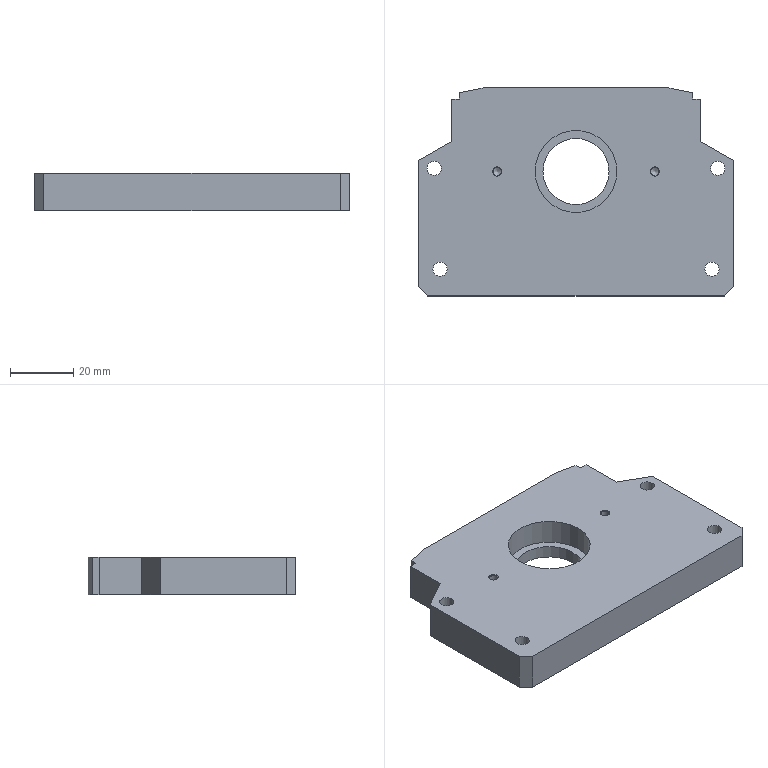Part | NX | 1 solid | 45 faces | box 100 x 66 x 12 mm | volume 66555 mm3 | plane 23 | cylinder 14 | cone 8 | commonest cylinder face diameters 2.5 x4 4.5 x4 8 x4 21 x1 26 x1
STEP:
#1=CARTESIAN_POINT('',(569.577,189.79,0.));
#2=VERTEX_POINT('',#1);
#3=CARTESIAN_POINT('',(559.077,189.79,0.));
#4=DIRECTION('',(0.,0.,-1.));
#5=DIRECTION('',(1.,0.,0.));
#6=AXIS2_PLACEMENT_3D('',#3,#4,#5);
#7=CIRCLE('',#6,10.5);
#8=EDGE_CURVE('',#2,#2,#7,.T.);
#9=ORIENTED_EDGE('',*,*,#8,.T.);
#10=EDGE_LOOP('',(#9));
#11=FACE_BOUND('',#10,.T.);
#12=CARTESIAN_POINT('',(569.577,189.79,4.));
#13=VERTEX_POINT('',#12);
#14=CARTESIAN_POINT('',(559.077,189.79,4.));
#15=DIRECTION('',(0.,0.,1.));
#16=DIRECTION('',(1.,0.,0.));
#17=AXIS2_PLACEMENT_3D('',#14,#15,#16);
#18=CIRCLE('',#17,10.5);
#19=EDGE_CURVE('',#13,#13,#18,.T.);
#20=ORIENTED_EDGE('',*,*,#19,.T.);
#21=EDGE_LOOP('',(#20));
#22=FACE_BOUND('',#21,.T.);
#23=CARTESIAN_POINT('',(559.077,189.79,0.));
#24=DIRECTION('',(0.,0.,1.));
#25=DIRECTION('',(-1.,0.,0.));
#26=AXIS2_PLACEMENT_3D('',#23,#24,#25);
#27=CYLINDRICAL_SURFACE('',#26,10.5);
#28=ADVANCED_FACE('',(#11,#22),#27,.F.);
#29=CARTESIAN_POINT('',(509.077,193.29,12.));
#30=VERTEX_POINT('',#29);
#31=CARTESIAN_POINT('',(509.077,153.29,12.));
#32=VERTEX_POINT('',#31);
#33=CARTESIAN_POINT('',(509.077,193.29,12.));
#34=DIRECTION('',(0.,-1.,0.));
#35=VECTOR('',#34,1.);
#36=LINE('',#33,#35);
#37=EDGE_CURVE('',#30,#32,#36,.T.);
#38=ORIENTED_EDGE('',*,*,#37,.F.);
#39=CARTESIAN_POINT('',(509.077,193.29,0.));
#40=VERTEX_POINT('',#39);
#41=CARTESIAN_POINT('',(509.077,193.29,0.));
#42=DIRECTION('',(0.,0.,1.));
#43=VECTOR('',#42,1.);
#44=LINE('',#41,#43);
#45=EDGE_CURVE('',#40,#30,#44,.T.);
#46=ORIENTED_EDGE('',*,*,#45,.F.);
#47=CARTESIAN_POINT('',(509.077,153.29,0.));
#48=VERTEX_POINT('',#47);
#49=CARTESIAN_POINT('',(509.077,193.29,0.));
#50=DIRECTION('',(0.,-1.,0.));
#51=VECTOR('',#50,1.);
#52=LINE('',#49,#51);
#53=EDGE_CURVE('',#40,#48,#52,.T.);
#54=ORIENTED_EDGE('',*,*,#53,.T.);
#55=CARTESIAN_POINT('',(509.077,153.29,0.));
#56=DIRECTION('',(0.,0.,1.));
#57=VECTOR('',#56,1.);
#58=LINE('',#55,#57);
#59=EDGE_CURVE('',#48,#32,#58,.T.);
#60=ORIENTED_EDGE('',*,*,#59,.T.);
#61=EDGE_LOOP('',(#38,#46,#54,#60));
#62=FACE_OUTER_BOUND('',#61,.T.);
#63=CARTESIAN_POINT('',(509.077,193.29,0.));
#64=DIRECTION('',(-1.,0.,0.));
#65=DIRECTION('',(0.,0.,-1.));
#66=AXIS2_PLACEMENT_3D('',#63,#64,#65);
#67=PLANE('',#66);
#68=ADVANCED_FACE('',(#62),#67,.T.);
#69=CARTESIAN_POINT('',(512.077,150.29,12.));
#70=VERTEX_POINT('',#69);
#71=CARTESIAN_POINT('',(509.077,153.29,12.));
#72=DIRECTION('',(0.7071,-0.7071,0.));
#73=VECTOR('',#72,1.);
#74=LINE('',#71,#73);
#75=EDGE_CURVE('',#32,#70,#74,.T.);
#76=ORIENTED_EDGE('',*,*,#75,.F.);
#77=ORIENTED_EDGE('',*,*,#59,.F.);
#78=CARTESIAN_POINT('',(512.077,150.29,0.));
#79=VERTEX_POINT('',#78);
#80=CARTESIAN_POINT('',(509.077,153.29,0.));
#81=DIRECTION('',(0.7071,-0.7071,0.));
#82=VECTOR('',#81,1.);
#83=LINE('',#80,#82);
#84=EDGE_CURVE('',#48,#79,#83,.T.);
#85=ORIENTED_EDGE('',*,*,#84,.T.);
#86=CARTESIAN_POINT('',(512.077,150.29,0.));
#87=DIRECTION('',(0.,0.,1.));
#88=VECTOR('',#87,1.);
#89=LINE('',#86,#88);
#90=EDGE_CURVE('',#79,#70,#89,.T.);
#91=ORIENTED_EDGE('',*,*,#90,.T.);
#92=EDGE_LOOP('',(#76,#77,#85,#91));
#93=FACE_OUTER_BOUND('',#92,.T.);
#94=CARTESIAN_POINT('',(509.077,153.29,0.));
#95=DIRECTION('',(-0.7071,-0.7071,0.));
#96=DIRECTION('',(-0.7071,0.7071,0.));
#97=AXIS2_PLACEMENT_3D('',#94,#95,#96);
#98=PLANE('',#97);
#99=ADVANCED_FACE('',(#93),#98,.T.);
#100=CARTESIAN_POINT('',(606.077,150.29,12.));
#101=VERTEX_POINT('',#100);
#102=CARTESIAN_POINT('',(512.077,150.29,12.));
#103=DIRECTION('',(1.,0.,0.));
#104=VECTOR('',#103,1.);
#105=LINE('',#102,#104);
#106=EDGE_CURVE('',#70,#101,#105,.T.);
#107=ORIENTED_EDGE('',*,*,#106,.F.);
#108=ORIENTED_EDGE('',*,*,#90,.F.);
#109=CARTESIAN_POINT('',(606.077,150.29,0.));
#110=VERTEX_POINT('',#109);
#111=CARTESIAN_POINT('',(512.077,150.29,0.));
#112=DIRECTION('',(1.,0.,0.));
#113=VECTOR('',#112,1.);
#114=LINE('',#111,#113);
#115=EDGE_CURVE('',#79,#110,#114,.T.);
#116=ORIENTED_EDGE('',*,*,#115,.T.);
#117=CARTESIAN_POINT('',(606.077,150.29,0.));
#118=DIRECTION('',(0.,0.,1.));
#119=VECTOR('',#118,1.);
#120=LINE('',#117,#119);
#121=EDGE_CURVE('',#110,#101,#120,.T.);
#122=ORIENTED_EDGE('',*,*,#121,.T.);
#123=EDGE_LOOP('',(#107,#108,#116,#122));
#124=FACE_OUTER_BOUND('',#123,.T.);
#125=CARTESIAN_POINT('',(512.077,150.29,0.));
#126=DIRECTION('',(0.,-1.,0.));
#127=DIRECTION('',(0.,0.,1.));
#128=AXIS2_PLACEMENT_3D('',#125,#126,#127);
#129=PLANE('',#128);
#130=ADVANCED_FACE('',(#124),#129,.T.);
#131=CARTESIAN_POINT('',(609.077,153.29,12.));
#132=VERTEX_POINT('',#131);
#133=CARTESIAN_POINT('',(606.077,150.29,12.));
#134=DIRECTION('',(0.7071,0.7071,0.));
#135=VECTOR('',#134,1.);
#136=LINE('',#133,#135);
#137=EDGE_CURVE('',#101,#132,#136,.T.);
#138=ORIENTED_EDGE('',*,*,#137,.F.);
#139=ORIENTED_EDGE('',*,*,#121,.F.);
#140=CARTESIAN_POINT('',(609.077,153.29,0.));
#141=VERTEX_POINT('',#140);
#142=CARTESIAN_POINT('',(606.077,150.29,0.));
#143=DIRECTION('',(0.7071,0.7071,0.));
#144=VECTOR('',#143,1.);
#145=LINE('',#142,#144);
#146=EDGE_CURVE('',#110,#141,#145,.T.);
#147=ORIENTED_EDGE('',*,*,#146,.T.);
#148=CARTESIAN_POINT('',(609.077,153.29,0.));
#149=DIRECTION('',(0.,0.,1.));
#150=VECTOR('',#149,1.);
#151=LINE('',#148,#150);
#152=EDGE_CURVE('',#141,#132,#151,.T.);
#153=ORIENTED_EDGE('',*,*,#152,.T.);
#154=EDGE_LOOP('',(#138,#139,#147,#153));
#155=FACE_OUTER_BOUND('',#154,.T.);
#156=CARTESIAN_POINT('',(606.077,150.29,0.));
#157=DIRECTION('',(0.7071,-0.7071,0.));
#158=DIRECTION('',(-0.7071,-0.7071,0.));
#159=AXIS2_PLACEMENT_3D('',#156,#157,#158);
#160=PLANE('',#159);
#161=ADVANCED_FACE('',(#155),#160,.T.);
#162=CARTESIAN_POINT('',(609.077,193.29,12.));
#163=VERTEX_POINT('',#162);
#164=CARTESIAN_POINT('',(609.077,153.29,12.));
#165=DIRECTION('',(0.,1.,0.));
#166=VECTOR('',#165,1.);
#167=LINE('',#164,#166);
#168=EDGE_CURVE('',#132,#163,#167,.T.);
#169=ORIENTED_EDGE('',*,*,#168,.F.);
#170=ORIENTED_EDGE('',*,*,#152,.F.);
#171=CARTESIAN_POINT('',(609.077,193.29,0.));
#172=VERTEX_POINT('',#171);
#173=CARTESIAN_POINT('',(609.077,153.29,0.));
#174=DIRECTION('',(0.,1.,0.));
#175=VECTOR('',#174,1.);
#176=LINE('',#173,#175);
#177=EDGE_CURVE('',#141,#172,#176,.T.);
#178=ORIENTED_EDGE('',*,*,#177,.T.);
#179=CARTESIAN_POINT('',(609.077,193.29,0.));
#180=DIRECTION('',(0.,0.,1.));
#181=VECTOR('',#180,1.);
#182=LINE('',#179,#181);
#183=EDGE_CURVE('',#172,#163,#182,.T.);
#184=ORIENTED_EDGE('',*,*,#183,.T.);
#185=EDGE_LOOP('',(#169,#170,#178,#184));
#186=FACE_OUTER_BOUND('',#185,.T.);
#187=CARTESIAN_POINT('',(609.077,153.29,0.));
#188=DIRECTION('',(1.,0.,0.));
#189=DIRECTION('',(0.,0.,1.));
#190=AXIS2_PLACEMENT_3D('',#187,#188,#189);
#191=PLANE('',#190);
#192=ADVANCED_FACE('',(#186),#191,.T.);
#193=CARTESIAN_POINT('',(598.577,199.29,12.));
#194=VERTEX_POINT('',#193);
#195=CARTESIAN_POINT('',(609.077,193.29,12.));
#196=DIRECTION('',(-0.8682,0.4961,0.));
#197=VECTOR('',#196,1.);
#198=LINE('',#195,#197);
#199=EDGE_CURVE('',#163,#194,#198,.T.);
#200=ORIENTED_EDGE('',*,*,#199,.F.);
#201=ORIENTED_EDGE('',*,*,#183,.F.);
#202=CARTESIAN_POINT('',(598.577,199.29,0.));
#203=VERTEX_POINT('',#202);
#204=CARTESIAN_POINT('',(609.077,193.29,0.));
#205=DIRECTION('',(-0.8682,0.4961,0.));
#206=VECTOR('',#205,1.);
#207=LINE('',#204,#206);
#208=EDGE_CURVE('',#172,#203,#207,.T.);
#209=ORIENTED_EDGE('',*,*,#208,.T.);
#210=CARTESIAN_POINT('',(598.577,199.29,0.));
#211=DIRECTION('',(0.,0.,1.));
#212=VECTOR('',#211,1.);
#213=LINE('',#210,#212);
#214=EDGE_CURVE('',#203,#194,#213,.T.);
#215=ORIENTED_EDGE('',*,*,#214,.T.);
#216=EDGE_LOOP('',(#200,#201,#209,#215));
#217=FACE_OUTER_BOUND('',#216,.T.);
#218=CARTESIAN_POINT('',(609.077,193.29,0.));
#219=DIRECTION('',(0.4961,0.8682,0.));
#220=DIRECTION('',(0.8682,-0.4961,0.));
#221=AXIS2_PLACEMENT_3D('',#218,#219,#220);
#222=PLANE('',#221);
#223=ADVANCED_FACE('',(#217),#222,.T.);
#224=CARTESIAN_POINT('',(598.577,212.79,12.));
#225=VERTEX_POINT('',#224);
#226=CARTESIAN_POINT('',(598.577,199.29,12.));
#227=DIRECTION('',(0.,1.,0.));
#228=VECTOR('',#227,1.);
#229=LINE('',#226,#228);
#230=EDGE_CURVE('',#194,#225,#229,.T.);
#231=ORIENTED_EDGE('',*,*,#230,.F.);
#232=ORIENTED_EDGE('',*,*,#214,.F.);
#233=CARTESIAN_POINT('',(598.577,212.79,0.));
#234=VERTEX_POINT('',#233);
#235=CARTESIAN_POINT('',(598.577,199.29,0.));
#236=DIRECTION('',(0.,1.,0.));
#237=VECTOR('',#236,1.);
#238=LINE('',#235,#237);
#239=EDGE_CURVE('',#203,#234,#238,.T.);
#240=ORIENTED_EDGE('',*,*,#239,.T.);
#241=CARTESIAN_POINT('',(598.577,212.79,0.));
#242=DIRECTION('',(0.,0.,1.));
#243=VECTOR('',#242,1.);
#244=LINE('',#241,#243);
#245=EDGE_CURVE('',#234,#225,#244,.T.);
#246=ORIENTED_EDGE('',*,*,#245,.T.);
#247=EDGE_LOOP('',(#231,#232,#240,#246));
#248=FACE_OUTER_BOUND('',#247,.T.);
#249=CARTESIAN_POINT('',(598.577,199.29,0.));
#250=DIRECTION('',(1.,0.,0.));
#251=DIRECTION('',(0.,0.,1.));
#252=AXIS2_PLACEMENT_3D('',#249,#250,#251);
#253=PLANE('',#252);
#254=ADVANCED_FACE('',(#248),#253,.T.);
#255=CARTESIAN_POINT('',(596.077,212.79,12.));
#256=VERTEX_POINT('',#255);
#257=CARTESIAN_POINT('',(598.577,212.79,12.));
#258=DIRECTION('',(-1.,0.,0.));
#259=VECTOR('',#258,1.);
#260=LINE('',#257,#259);
#261=EDGE_CURVE('',#225,#256,#260,.T.);
#262=ORIENTED_EDGE('',*,*,#261,.F.);
#263=ORIENTED_EDGE('',*,*,#245,.F.);
#264=CARTESIAN_POINT('',(596.077,212.79,0.));
#265=VERTEX_POINT('',#264);
#266=CARTESIAN_POINT('',(598.577,212.79,0.));
#267=DIRECTION('',(-1.,0.,0.));
#268=VECTOR('',#267,1.);
#269=LINE('',#266,#268);
#270=EDGE_CURVE('',#234,#265,#269,.T.);
#271=ORIENTED_EDGE('',*,*,#270,.T.);
#272=CARTESIAN_POINT('',(596.077,212.79,0.));
#273=DIRECTION('',(0.,0.,1.));
#274=VECTOR('',#273,1.);
#275=LINE('',#272,#274);
#276=EDGE_CURVE('',#265,#256,#275,.T.);
#277=ORIENTED_EDGE('',*,*,#276,.T.);
#278=EDGE_LOOP('',(#262,#263,#271,#277));
#279=FACE_OUTER_BOUND('',#278,.T.);
#280=CARTESIAN_POINT('',(598.577,212.79,0.));
#281=DIRECTION('',(0.,1.,0.));
#282=DIRECTION('',(0.,0.,-1.));
#283=AXIS2_PLACEMENT_3D('',#280,#281,#282);
#284=PLANE('',#283);
#285=ADVANCED_FACE('',(#279),#284,.T.);
#286=CARTESIAN_POINT('',(596.077,214.79,12.));
#287=VERTEX_POINT('',#286);
#288=CARTESIAN_POINT('',(596.077,212.79,12.));
#289=DIRECTION('',(0.,1.,0.));
#290=VECTOR('',#289,1.);
#291=LINE('',#288,#290);
#292=EDGE_CURVE('',#256,#287,#291,.T.);
#293=ORIENTED_EDGE('',*,*,#292,.F.);
#294=ORIENTED_EDGE('',*,*,#276,.F.);
#295=CARTESIAN_POINT('',(596.077,214.79,0.));
#296=VERTEX_POINT('',#295);
#297=CARTESIAN_POINT('',(596.077,212.79,0.));
#298=DIRECTION('',(0.,1.,0.));
#299=VECTOR('',#298,1.);
#300=LINE('',#297,#299);
#301=EDGE_CURVE('',#265,#296,#300,.T.);
#302=ORIENTED_EDGE('',*,*,#301,.T.);
#303=CARTESIAN_POINT('',(596.077,214.79,0.));
#304=DIRECTION('',(0.,0.,1.));
#305=VECTOR('',#304,1.);
#306=LINE('',#303,#305);
#307=EDGE_CURVE('',#296,#287,#306,.T.);
#308=ORIENTED_EDGE('',*,*,#307,.T.);
#309=EDGE_LOOP('',(#293,#294,#302,#308));
#310=FACE_OUTER_BOUND('',#309,.T.);
#311=CARTESIAN_POINT('',(596.077,212.79,0.));
#312=DIRECTION('',(1.,0.,0.));
#313=DIRECTION('',(0.,0.,1.));
#314=AXIS2_PLACEMENT_3D('',#311,#312,#313);
#315=PLANE('',#314);
#316=ADVANCED_FACE('',(#310),#315,.T.);
#317=CARTESIAN_POINT('',(588.577,216.29,12.));
#318=VERTEX_POINT('',#317);
#319=CARTESIAN_POINT('',(596.077,214.79,12.));
#320=DIRECTION('',(-0.9806,0.1961,0.));
#321=VECTOR('',#320,1.);
#322=LINE('',#319,#321);
#323=EDGE_CURVE('',#287,#318,#322,.T.);
#324=ORIENTED_EDGE('',*,*,#323,.F.);
#325=ORIENTED_EDGE('',*,*,#307,.F.);
#326=CARTESIAN_POINT('',(588.577,216.29,0.));
#327=VERTEX_POINT('',#326);
#328=CARTESIAN_POINT('',(596.077,214.79,0.));
#329=DIRECTION('',(-0.9806,0.1961,0.));
#330=VECTOR('',#329,1.);
#331=LINE('',#328,#330);
#332=EDGE_CURVE('',#296,#327,#331,.T.);
#333=ORIENTED_EDGE('',*,*,#332,.T.);
#334=CARTESIAN_POINT('',(588.577,216.29,0.));
#335=DIRECTION('',(0.,0.,1.));
#336=VECTOR('',#335,1.);
#337=LINE('',#334,#336);
#338=EDGE_CURVE('',#327,#318,#337,.T.);
#339=ORIENTED_EDGE('',*,*,#338,.T.);
#340=EDGE_LOOP('',(#324,#325,#333,#339));
#341=FACE_OUTER_BOUND('',#340,.T.);
#342=CARTESIAN_POINT('',(596.077,214.79,0.));
#343=DIRECTION('',(0.1961,0.9806,0.));
#344=DIRECTION('',(0.9806,-0.1961,0.));
#345=AXIS2_PLACEMENT_3D('',#342,#343,#344);
#346=PLANE('',#345);
#347=ADVANCED_FACE('',(#341),#346,.T.);
#348=CARTESIAN_POINT('',(585.077,216.29,7.5));
#349=VERTEX_POINT('',#348);
#350=CARTESIAN_POINT('',(585.077,216.29,6.));
#351=DIRECTION('',(0.,-1.,0.));
#352=DIRECTION('',(0.,0.,1.));
#353=AXIS2_PLACEMENT_3D('',#350,#351,#352);
#354=CIRCLE('',#353,1.5);
#355=EDGE_CURVE('',#349,#349,#354,.T.);
#356=ORIENTED_EDGE('',*,*,#355,.T.);
#357=EDGE_LOOP('',(#356));
#358=FACE_BOUND('',#357,.T.);
#359=CARTESIAN_POINT('',(533.077,216.29,7.5));
#360=VERTEX_POINT('',#359);
#361=CARTESIAN_POINT('',(533.077,216.29,6.));
#362=DIRECTION('',(0.,-1.,0.));
#363=DIRECTION('',(0.,0.,1.));
#364=AXIS2_PLACEMENT_3D('',#361,#362,#363);
#365=CIRCLE('',#364,1.5);
#366=EDGE_CURVE('',#360,#360,#365,.T.);
#367=ORIENTED_EDGE('',*,*,#366,.T.);
#368=EDGE_LOOP('',(#367));
#369=FACE_BOUND('',#368,.T.);
#370=CARTESIAN_POINT('',(529.577,216.29,12.));
#371=VERTEX_POINT('',#370);
#372=CARTESIAN_POINT('',(588.577,216.29,12.));
#373=DIRECTION('',(-1.,0.,0.));
#374=VECTOR('',#373,1.);
#375=LINE('',#372,#374);
#376=EDGE_CURVE('',#318,#371,#375,.T.);
#377=ORIENTED_EDGE('',*,*,#376,.F.);
#378=ORIENTED_EDGE('',*,*,#338,.F.);
#379=CARTESIAN_POINT('',(529.577,216.29,0.));
#380=VERTEX_POINT('',#379);
#381=CARTESIAN_POINT('',(588.577,216.29,0.));
#382=DIRECTION('',(-1.,0.,0.));
#383=VECTOR('',#382,1.);
#384=LINE('',#381,#383);
#385=EDGE_CURVE('',#327,#380,#384,.T.);
#386=ORIENTED_EDGE('',*,*,#385,.T.);
#387=CARTESIAN_POINT('',(529.577,216.29,0.));
#388=DIRECTION('',(0.,0.,1.));
#389=VECTOR('',#388,1.);
#390=LINE('',#387,#389);
#391=EDGE_CURVE('',#380,#371,#390,.T.);
#392=ORIENTED_EDGE('',*,*,#391,.T.);
#393=EDGE_LOOP('',(#377,#378,#386,#392));
#394=FACE_BOUND('',#393,.T.);
#395=CARTESIAN_POINT('',(588.577,216.29,0.));
#396=DIRECTION('',(0.,1.,0.));
#397=DIRECTION('',(0.,0.,-1.));
#398=AXIS2_PLACEMENT_3D('',#395,#396,#397);
#399=PLANE('',#398);
#400=ADVANCED_FACE('',(#358,#369,#394),#399,.T.);
#401=CARTESIAN_POINT('',(522.077,214.79,12.));
#402=VERTEX_POINT('',#401);
#403=CARTESIAN_POINT('',(529.577,216.29,12.));
#404=DIRECTION('',(-0.9806,-0.1961,0.));
#405=VECTOR('',#404,1.);
#406=LINE('',#403,#405);
#407=EDGE_CURVE('',#371,#402,#406,.T.);
#408=ORIENTED_EDGE('',*,*,#407,.F.);
#409=ORIENTED_EDGE('',*,*,#391,.F.);
#410=CARTESIAN_POINT('',(522.077,214.79,0.));
#411=VERTEX_POINT('',#410);
#412=CARTESIAN_POINT('',(529.577,216.29,0.));
#413=DIRECTION('',(-0.9806,-0.1961,0.));
#414=VECTOR('',#413,1.);
#415=LINE('',#412,#414);
#416=EDGE_CURVE('',#380,#411,#415,.T.);
#417=ORIENTED_EDGE('',*,*,#416,.T.);
#418=CARTESIAN_POINT('',(522.077,214.79,0.));
#419=DIRECTION('',(0.,0.,1.));
#420=VECTOR('',#419,1.);
#421=LINE('',#418,#420);
#422=EDGE_CURVE('',#411,#402,#421,.T.);
#423=ORIENTED_EDGE('',*,*,#422,.T.);
#424=EDGE_LOOP('',(#408,#409,#417,#423));
#425=FACE_OUTER_BOUND('',#424,.T.);
#426=CARTESIAN_POINT('',(529.577,216.29,0.));
#427=DIRECTION('',(-0.1961,0.9806,0.));
#428=DIRECTION('',(0.9806,0.1961,0.));
#429=AXIS2_PLACEMENT_3D('',#426,#427,#428);
#430=PLANE('',#429);
#431=ADVANCED_FACE('',(#425),#430,.T.);
#432=CARTESIAN_POINT('',(522.077,212.79,12.));
#433=VERTEX_POINT('',#432);
#434=CARTESIAN_POINT('',(522.077,214.79,12.));
#435=DIRECTION('',(0.,-1.,0.));
#436=VECTOR('',#435,1.);
#437=LINE('',#434,#436);
#438=EDGE_CURVE('',#402,#433,#437,.T.);
#439=ORIENTED_EDGE('',*,*,#438,.F.);
#440=ORIENTED_EDGE('',*,*,#422,.F.);
#441=CARTESIAN_POINT('',(522.077,212.79,0.));
#442=VERTEX_POINT('',#441);
#443=CARTESIAN_POINT('',(522.077,214.79,0.));
#444=DIRECTION('',(0.,-1.,0.));
#445=VECTOR('',#444,1.);
#446=LINE('',#443,#445);
#447=EDGE_CURVE('',#411,#442,#446,.T.);
#448=ORIENTED_EDGE('',*,*,#447,.T.);
#449=CARTESIAN_POINT('',(522.077,212.79,0.));
#450=DIRECTION('',(0.,0.,1.));
#451=VECTOR('',#450,1.);
#452=LINE('',#449,#451);
#453=EDGE_CURVE('',#442,#433,#452,.T.);
#454=ORIENTED_EDGE('',*,*,#453,.T.);
#455=EDGE_LOOP('',(#439,#440,#448,#454));
#456=FACE_OUTER_BOUND('',#455,.T.);
#457=CARTESIAN_POINT('',(522.077,214.79,0.));
#458=DIRECTION('',(-1.,0.,0.));
#459=DIRECTION('',(0.,0.,-1.));
#460=AXIS2_PLACEMENT_3D('',#457,#458,#459);
#461=PLANE('',#460);
#462=ADVANCED_FACE('',(#456),#461,.T.);
#463=CARTESIAN_POINT('',(519.577,212.79,12.));
#464=VERTEX_POINT('',#463);
#465=CARTESIAN_POINT('',(522.077,212.79,12.));
#466=DIRECTION('',(-1.,0.,0.));
#467=VECTOR('',#466,1.);
#468=LINE('',#465,#467);
#469=EDGE_CURVE('',#433,#464,#468,.T.);
#470=ORIENTED_EDGE('',*,*,#469,.F.);
#471=ORIENTED_EDGE('',*,*,#453,.F.);
#472=CARTESIAN_POINT('',(519.577,212.79,0.));
#473=VERTEX_POINT('',#472);
#474=CARTESIAN_POINT('',(522.077,212.79,0.));
#475=DIRECTION('',(-1.,0.,0.));
#476=VECTOR('',#475,1.);
#477=LINE('',#474,#476);
#478=EDGE_CURVE('',#442,#473,#477,.T.);
#479=ORIENTED_EDGE('',*,*,#478,.T.);
#480=CARTESIAN_POINT('',(519.577,212.79,0.));
#481=DIRECTION('',(0.,0.,1.));
#482=VECTOR('',#481,1.);
#483=LINE('',#480,#482);
#484=EDGE_CURVE('',#473,#464,#483,.T.);
#485=ORIENTED_EDGE('',*,*,#484,.T.);
#486=EDGE_LOOP('',(#470,#471,#479,#485));
#487=FACE_OUTER_BOUND('',#486,.T.);
#488=CARTESIAN_POINT('',(522.077,212.79,0.));
#489=DIRECTION('',(0.,1.,0.));
#490=DIRECTION('',(0.,0.,-1.));
#491=AXIS2_PLACEMENT_3D('',#488,#489,#490);
#492=PLANE('',#491);
#493=ADVANCED_FACE('',(#487),#492,.T.);
#494=CARTESIAN_POINT('',(519.577,199.29,12.));
#495=VERTEX_POINT('',#494);
#496=CARTESIAN_POINT('',(519.577,212.79,12.));
#497=DIRECTION('',(0.,-1.,0.));
#498=VECTOR('',#497,1.);
#499=LINE('',#496,#498);
#500=EDGE_CURVE('',#464,#495,#499,.T.);
#501=ORIENTED_EDGE('',*,*,#500,.F.);
#502=ORIENTED_EDGE('',*,*,#484,.F.);
#503=CARTESIAN_POINT('',(519.577,199.29,0.));
#504=VERTEX_POINT('',#503);
#505=CARTESIAN_POINT('',(519.577,212.79,0.));
#506=DIRECTION('',(0.,-1.,0.));
#507=VECTOR('',#506,1.);
#508=LINE('',#505,#507);
#509=EDGE_CURVE('',#473,#504,#508,.T.);
#510=ORIENTED_EDGE('',*,*,#509,.T.);
#511=CARTESIAN_POINT('',(519.577,199.29,0.));
#512=DIRECTION('',(0.,0.,1.));
#513=VECTOR('',#512,1.);
#514=LINE('',#511,#513);
#515=EDGE_CURVE('',#504,#495,#514,.T.);
#516=ORIENTED_EDGE('',*,*,#515,.T.);
#517=EDGE_LOOP('',(#501,#502,#510,#516));
#518=FACE_OUTER_BOUND('',#517,.T.);
#519=CARTESIAN_POINT('',(519.577,212.79,0.));
#520=DIRECTION('',(-1.,0.,0.));
#521=DIRECTION('',(0.,0.,-1.));
#522=AXIS2_PLACEMENT_3D('',#519,#520,#521);
#523=PLANE('',#522);
#524=ADVANCED_FACE('',(#518),#523,.T.);
#525=CARTESIAN_POINT('',(604.477,158.79,4.6));
#526=VERTEX_POINT('',#525);
#527=CARTESIAN_POINT('',(602.227,158.79,4.6));
#528=DIRECTION('',(0.,0.,1.));
#529=DIRECTION('',(1.,0.,0.));
#530=AXIS2_PLACEMENT_3D('',#527,#528,#529);
#531=CIRCLE('',#530,2.25);
#532=EDGE_CURVE('',#526,#526,#531,.T.);
#533=ORIENTED_EDGE('',*,*,#532,.F.);
#534=EDGE_LOOP('',(#533));
#535=FACE_BOUND('',#534,.T.);
#536=CARTESIAN_POINT('',(599.977,158.79,12.));
#537=VERTEX_POINT('',#536);
#538=CARTESIAN_POINT('',(602.227,158.79,12.));
#539=DIRECTION('',(0.,0.,-1.));
#540=DIRECTION('',(-1.,0.,0.));
#541=AXIS2_PLACEMENT_3D('',#538,#539,#540);
#542=CIRCLE('',#541,2.25);
#543=EDGE_CURVE('',#537,#537,#542,.T.);
#544=ORIENTED_EDGE('',*,*,#543,.F.);
#545=EDGE_LOOP('',(#544));
#546=FACE_BOUND('',#545,.T.);
#547=CARTESIAN_POINT('',(602.227,158.79,0.));
#548=DIRECTION('',(0.,0.,1.));
#549=DIRECTION('',(-1.,0.,0.));
#550=AXIS2_PLACEMENT_3D('',#547,#548,#549);
#551=CYLINDRICAL_SURFACE('',#550,2.25);
#552=ADVANCED_FACE('',(#535,#546),#551,.F.);
#553=CARTESIAN_POINT('',(518.177,158.79,4.6));
#554=VERTEX_POINT('',#553);
#555=CARTESIAN_POINT('',(515.927,158.79,4.6));
#556=DIRECTION('',(0.,0.,1.));
#557=DIRECTION('',(1.,0.,0.));
#558=AXIS2_PLACEMENT_3D('',#555,#556,#557);
#559=CIRCLE('',#558,2.25);
#560=EDGE_CURVE('',#554,#554,#559,.T.);
#561=ORIENTED_EDGE('',*,*,#560,.F.);
#562=EDGE_LOOP('',(#561));
#563=FACE_BOUND('',#562,.T.);
#564=CARTESIAN_POINT('',(513.677,158.79,12.));
#565=VERTEX_POINT('',#564);
#566=CARTESIAN_POINT('',(515.927,158.79,12.));
#567=DIRECTION('',(0.,0.,-1.));
#568=DIRECTION('',(-1.,0.,0.));
#569=AXIS2_PLACEMENT_3D('',#566,#567,#568);
#570=CIRCLE('',#569,2.25);
#571=EDGE_CURVE('',#565,#565,#570,.T.);
#572=ORIENTED_EDGE('',*,*,#571,.F.);
#573=EDGE_LOOP('',(#572));
#574=FACE_BOUND('',#573,.T.);
#575=CARTESIAN_POINT('',(515.927,158.79,0.));
#576=DIRECTION('',(0.,0.,1.));
#577=DIRECTION('',(-1.,0.,0.));
#578=AXIS2_PLACEMENT_3D('',#575,#576,#577);
#579=CYLINDRICAL_SURFACE('',#578,2.25);
#580=ADVANCED_FACE('',(#563,#574),#579,.F.);
#581=CARTESIAN_POINT('',(516.327,190.79,4.6));
#582=VERTEX_POINT('',#581);
#583=CARTESIAN_POINT('',(514.077,190.79,4.6));
#584=DIRECTION('',(0.,0.,1.));
#585=DIRECTION('',(1.,0.,0.));
#586=AXIS2_PLACEMENT_3D('',#583,#584,#585);
#587=CIRCLE('',#586,2.25);
#588=EDGE_CURVE('',#582,#582,#587,.T.);
#589=ORIENTED_EDGE('',*,*,#588,.F.);
#590=EDGE_LOOP('',(#589));
#591=FACE_BOUND('',#590,.T.);
#592=CARTESIAN_POINT('',(511.827,190.79,12.));
#593=VERTEX_POINT('',#592);
#594=CARTESIAN_POINT('',(514.077,190.79,12.));
#595=DIRECTION('',(0.,0.,-1.));
#596=DIRECTION('',(-1.,0.,0.));
#597=AXIS2_PLACEMENT_3D('',#594,#595,#596);
#598=CIRCLE('',#597,2.25);
#599=EDGE_CURVE('',#593,#593,#598,.T.);
#600=ORIENTED_EDGE('',*,*,#599,.F.);
#601=EDGE_LOOP('',(#600));
#602=FACE_BOUND('',#601,.T.);
#603=CARTESIAN_POINT('',(514.077,190.79,0.));
#604=DIRECTION('',(0.,0.,1.));
#605=DIRECTION('',(-1.,0.,0.));
#606=AXIS2_PLACEMENT_3D('',#603,#604,#605);
#607=CYLINDRICAL_SURFACE('',#606,2.25);
#608=ADVANCED_FACE('',(#591,#602),#607,.F.);
#609=CARTESIAN_POINT('',(519.577,199.29,12.));
#610=DIRECTION('',(-0.8682,-0.4961,0.));
#611=VECTOR('',#610,1.);
#612=LINE('',#609,#611);
#613=EDGE_CURVE('',#495,#30,#612,.T.);
#614=ORIENTED_EDGE('',*,*,#613,.F.);
#615=ORIENTED_EDGE('',*,*,#515,.F.);
#616=CARTESIAN_POINT('',(519.577,199.29,0.));
#617=DIRECTION('',(-0.8682,-0.4961,0.));
#618=VECTOR('',#617,1.);
#619=LINE('',#616,#618);
#620=EDGE_CURVE('',#504,#40,#619,.T.);
#621=ORIENTED_EDGE('',*,*,#620,.T.);
#622=ORIENTED_EDGE('',*,*,#45,.T.);
#623=EDGE_LOOP('',(#614,#615,#621,#622));
#624=FACE_OUTER_BOUND('',#623,.T.);
#625=CARTESIAN_POINT('',(519.577,199.29,0.));
#626=DIRECTION('',(-0.4961,0.8682,0.));
#627=DIRECTION('',(0.8682,0.4961,0.));
#628=AXIS2_PLACEMENT_3D('',#625,#626,#627);
#629=PLANE('',#628);
#630=ADVANCED_FACE('',(#624),#629,.T.);
#631=CARTESIAN_POINT('',(606.327,190.79,4.6));
#632=VERTEX_POINT('',#631);
#633=CARTESIAN_POINT('',(604.077,190.79,4.6));
#634=DIRECTION('',(0.,0.,1.));
#635=DIRECTION('',(1.,0.,0.));
#636=AXIS2_PLACEMENT_3D('',#633,#634,#635);
#637=CIRCLE('',#636,2.25);
#638=EDGE_CURVE('',#632,#632,#637,.T.);
#639=ORIENTED_EDGE('',*,*,#638,.F.);
#640=EDGE_LOOP('',(#639));
#641=FACE_BOUND('',#640,.T.);
#642=CARTESIAN_POINT('',(601.827,190.79,12.));
#643=VERTEX_POINT('',#642);
#644=CARTESIAN_POINT('',(604.077,190.79,12.));
#645=DIRECTION('',(0.,0.,-1.));
#646=DIRECTION('',(-1.,0.,0.));
#647=AXIS2_PLACEMENT_3D('',#644,#645,#646);
#648=CIRCLE('',#647,2.25);
#649=EDGE_CURVE('',#643,#643,#648,.T.);
#650=ORIENTED_EDGE('',*,*,#649,.F.);
#651=EDGE_LOOP('',(#650));
#652=FACE_BOUND('',#651,.T.);
#653=CARTESIAN_POINT('',(604.077,190.79,0.));
#654=DIRECTION('',(0.,0.,1.));
#655=DIRECTION('',(-1.,0.,0.));
#656=AXIS2_PLACEMENT_3D('',#653,#654,#655);
#657=CYLINDRICAL_SURFACE('',#656,2.25);
#658=ADVANCED_FACE('',(#641,#652),#657,.F.);
#659=CARTESIAN_POINT('',(606.227,158.79,0.));
#660=VERTEX_POINT('',#659);
#661=CARTESIAN_POINT('',(602.227,158.79,0.));
#662=DIRECTION('',(0.,0.,1.));
#663=DIRECTION('',(1.,0.,0.));
#664=AXIS2_PLACEMENT_3D('',#661,#662,#663);
#665=CIRCLE('',#664,4.);
#666=EDGE_CURVE('',#660,#660,#665,.T.);
#667=ORIENTED_EDGE('',*,*,#666,.T.);
#668=EDGE_LOOP('',(#667));
#669=FACE_BOUND('',#668,.T.);
#670=CARTESIAN_POINT('',(519.927,158.79,0.));
#671=VERTEX_POINT('',#670);
#672=CARTESIAN_POINT('',(515.927,158.79,0.));
#673=DIRECTION('',(0.,0.,1.));
#674=DIRECTION('',(1.,0.,0.));
#675=AXIS2_PLACEMENT_3D('',#672,#673,#674);
#676=CIRCLE('',#675,4.);
#677=EDGE_CURVE('',#671,#671,#676,.T.);
#678=ORIENTED_EDGE('',*,*,#677,.T.);
#679=EDGE_LOOP('',(#678));
#680=FACE_BOUND('',#679,.T.);
#681=CARTESIAN_POINT('',(518.077,190.79,0.));
#682=VERTEX_POINT('',#681);
#683=CARTESIAN_POINT('',(514.077,190.79,0.));
#684=DIRECTION('',(0.,0.,1.));
#685=DIRECTION('',(1.,0.,0.));
#686=AXIS2_PLACEMENT_3D('',#683,#684,#685);
#687=CIRCLE('',#686,4.);
#688=EDGE_CURVE('',#682,#682,#687,.T.);
#689=ORIENTED_EDGE('',*,*,#688,.T.);
#690=EDGE_LOOP('',(#689));
#691=FACE_BOUND('',#690,.T.);
#692=CARTESIAN_POINT('',(608.077,190.79,0.));
#693=VERTEX_POINT('',#692);
#694=CARTESIAN_POINT('',(604.077,190.79,0.));
#695=DIRECTION('',(0.,0.,1.));
#696=DIRECTION('',(1.,0.,0.));
#697=AXIS2_PLACEMENT_3D('',#694,#695,#696);
#698=CIRCLE('',#697,4.);
#699=EDGE_CURVE('',#693,#693,#698,.T.);
#700=ORIENTED_EDGE('',*,*,#699,.T.);
#701=EDGE_LOOP('',(#700));
#702=FACE_BOUND('',#701,.T.);
#703=ORIENTED_EDGE('',*,*,#53,.F.);
#704=ORIENTED_EDGE('',*,*,#620,.F.);
#705=ORIENTED_EDGE('',*,*,#509,.F.);
#706=ORIENTED_EDGE('',*,*,#478,.F.);
#707=ORIENTED_EDGE('',*,*,#447,.F.);
#708=ORIENTED_EDGE('',*,*,#416,.F.);
#709=ORIENTED_EDGE('',*,*,#385,.F.);
#710=ORIENTED_EDGE('',*,*,#332,.F.);
#711=ORIENTED_EDGE('',*,*,#301,.F.);
#712=ORIENTED_EDGE('',*,*,#270,.F.);
#713=ORIENTED_EDGE('',*,*,#239,.F.);
#714=ORIENTED_EDGE('',*,*,#208,.F.);
#715=ORIENTED_EDGE('',*,*,#177,.F.);
#716=ORIENTED_EDGE('',*,*,#146,.F.);
#717=ORIENTED_EDGE('',*,*,#115,.F.);
#718=ORIENTED_EDGE('',*,*,#84,.F.);
#719=EDGE_LOOP('',(#703,#704,#705,#706,#707,#708,#709,#710,#711,#712,#713,#714,#715,#716,#717,#718));
#720=FACE_BOUND('',#719,.T.);
#721=ORIENTED_EDGE('',*,*,#8,.F.);
#722=EDGE_LOOP('',(#721));
#723=FACE_BOUND('',#722,.T.);
#724=CARTESIAN_POINT('',(514.077,190.79,0.));
#725=DIRECTION('',(0.,0.,-1.));
#726=DIRECTION('',(1.,0.,0.));
#727=AXIS2_PLACEMENT_3D('',#724,#725,#726);
#728=PLANE('',#727);
#729=ADVANCED_FACE('',(#669,#680,#691,#702,#720,#723),#728,.T.);
#730=CARTESIAN_POINT('',(582.577,189.79,12.));
#731=VERTEX_POINT('',#730);
#732=CARTESIAN_POINT('',(584.077,189.79,12.));
#733=DIRECTION('',(0.,0.,-1.));
#734=DIRECTION('',(-1.,0.,0.));
#735=AXIS2_PLACEMENT_3D('',#732,#733,#734);
#736=CIRCLE('',#735,1.5);
#737=EDGE_CURVE('',#731,#731,#736,.T.);
#738=ORIENTED_EDGE('',*,*,#737,.T.);
#739=EDGE_LOOP('',(#738));
#740=FACE_BOUND('',#739,.T.);
#741=CARTESIAN_POINT('',(532.577,189.79,12.));
#742=VERTEX_POINT('',#741);
#743=CARTESIAN_POINT('',(534.077,189.79,12.));
#744=DIRECTION('',(0.,0.,-1.));
#745=DIRECTION('',(-1.,0.,0.));
#746=AXIS2_PLACEMENT_3D('',#743,#744,#745);
#747=CIRCLE('',#746,1.5);
#748=EDGE_CURVE('',#742,#742,#747,.T.);
#749=ORIENTED_EDGE('',*,*,#748,.T.);
#750=EDGE_LOOP('',(#749));
#751=FACE_BOUND('',#750,.T.);
#752=CARTESIAN_POINT('',(572.077,189.79,12.));
#753=VERTEX_POINT('',#752);
#754=CARTESIAN_POINT('',(559.077,189.79,12.));
#755=DIRECTION('',(0.,0.,1.));
#756=DIRECTION('',(1.,0.,0.));
#757=AXIS2_PLACEMENT_3D('',#754,#755,#756);
#758=CIRCLE('',#757,13.);
#759=EDGE_CURVE('',#753,#753,#758,.T.);
#760=ORIENTED_EDGE('',*,*,#759,.F.);
#761=EDGE_LOOP('',(#760));
#762=FACE_BOUND('',#761,.T.);
#763=ORIENTED_EDGE('',*,*,#37,.T.);
#764=ORIENTED_EDGE('',*,*,#75,.T.);
#765=ORIENTED_EDGE('',*,*,#106,.T.);
#766=ORIENTED_EDGE('',*,*,#137,.T.);
#767=ORIENTED_EDGE('',*,*,#168,.T.);
#768=ORIENTED_EDGE('',*,*,#199,.T.);
#769=ORIENTED_EDGE('',*,*,#230,.T.);
#770=ORIENTED_EDGE('',*,*,#261,.T.);
#771=ORIENTED_EDGE('',*,*,#292,.T.);
#772=ORIENTED_EDGE('',*,*,#323,.T.);
#773=ORIENTED_EDGE('',*,*,#376,.T.);
#774=ORIENTED_EDGE('',*,*,#407,.T.);
#775=ORIENTED_EDGE('',*,*,#438,.T.);
#776=ORIENTED_EDGE('',*,*,#469,.T.);
#777=ORIENTED_EDGE('',*,*,#500,.T.);
#778=ORIENTED_EDGE('',*,*,#613,.T.);
#779=EDGE_LOOP('',(#763,#764,#765,#766,#767,#768,#769,#770,#771,#772,#773,#774,#775,#776,#777,#778));
#780=FACE_BOUND('',#779,.T.);
#781=ORIENTED_EDGE('',*,*,#599,.T.);
#782=EDGE_LOOP('',(#781));
#783=FACE_BOUND('',#782,.T.);
#784=ORIENTED_EDGE('',*,*,#571,.T.);
#785=EDGE_LOOP('',(#784));
#786=FACE_BOUND('',#785,.T.);
#787=ORIENTED_EDGE('',*,*,#543,.T.);
#788=EDGE_LOOP('',(#787));
#789=FACE_BOUND('',#788,.T.);
#790=ORIENTED_EDGE('',*,*,#649,.T.);
#791=EDGE_LOOP('',(#790));
#792=FACE_BOUND('',#791,.T.);
#793=CARTESIAN_POINT('',(514.077,190.79,12.));
#794=DIRECTION('',(0.,0.,-1.));
#795=DIRECTION('',(1.,0.,0.));
#796=AXIS2_PLACEMENT_3D('',#793,#794,#795);
#797=PLANE('',#796);
#798=ADVANCED_FACE('',(#740,#751,#762,#780,#783,#786,#789,#792),#797,.F.);
#799=ORIENTED_EDGE('',*,*,#759,.T.);
#800=EDGE_LOOP('',(#799));
#801=FACE_BOUND('',#800,.T.);
#802=CARTESIAN_POINT('',(572.077,189.79,4.));
#803=VERTEX_POINT('',#802);
#804=CARTESIAN_POINT('',(559.077,189.79,4.));
#805=DIRECTION('',(0.,0.,-1.));
#806=DIRECTION('',(1.,0.,0.));
#807=AXIS2_PLACEMENT_3D('',#804,#805,#806);
#808=CIRCLE('',#807,13.);
#809=EDGE_CURVE('',#803,#803,#808,.T.);
#810=ORIENTED_EDGE('',*,*,#809,.T.);
#811=EDGE_LOOP('',(#810));
#812=FACE_BOUND('',#811,.T.);
#813=CARTESIAN_POINT('',(559.077,189.79,4.));
#814=DIRECTION('',(0.,0.,1.));
#815=DIRECTION('',(-1.,0.,0.));
#816=AXIS2_PLACEMENT_3D('',#813,#814,#815);
#817=CYLINDRICAL_SURFACE('',#816,13.);
#818=ADVANCED_FACE('',(#801,#812),#817,.F.);
#819=ORIENTED_EDGE('',*,*,#19,.F.);
#820=EDGE_LOOP('',(#819));
#821=FACE_BOUND('',#820,.T.);
#822=ORIENTED_EDGE('',*,*,#809,.F.);
#823=EDGE_LOOP('',(#822));
#824=FACE_BOUND('',#823,.T.);
#825=CARTESIAN_POINT('',(559.077,189.79,4.));
#826=DIRECTION('',(0.,0.,1.));
#827=DIRECTION('',(-1.,0.,0.));
#828=AXIS2_PLACEMENT_3D('',#825,#826,#827);
#829=PLANE('',#828);
#830=ADVANCED_FACE('',(#821,#824),#829,.T.);
#831=CARTESIAN_POINT('',(532.827,189.79,6.));
#832=VERTEX_POINT('',#831);
#833=CARTESIAN_POINT('',(534.077,189.79,6.));
#834=DIRECTION('',(0.,0.,1.));
#835=DIRECTION('',(-1.,0.,0.));
#836=AXIS2_PLACEMENT_3D('',#833,#834,#835);
#837=CIRCLE('',#836,1.25);
#838=EDGE_CURVE('',#832,#832,#837,.T.);
#839=ORIENTED_EDGE('',*,*,#838,.T.);
#840=EDGE_LOOP('',(#839));
#841=FACE_BOUND('',#840,.T.);
#842=CARTESIAN_POINT('',(534.077,189.79,5.249));
#843=VERTEX_POINT('',#842);
#844=VERTEX_LOOP('',#843);
#845=FACE_BOUND('',#844,.T.);
#846=CARTESIAN_POINT('',(534.077,189.79,6.));
#847=DIRECTION('',(0.,0.,1.));
#848=DIRECTION('',(-1.,0.,0.));
#849=AXIS2_PLACEMENT_3D('',#846,#847,#848);
#850=CONICAL_SURFACE('',#849,1.25,59.);
#851=ADVANCED_FACE('',(#841,#845),#850,.F.);
#852=CARTESIAN_POINT('',(532.827,189.79,11.75));
#853=VERTEX_POINT('',#852);
#854=CARTESIAN_POINT('',(534.077,189.79,11.75));
#855=DIRECTION('',(0.,0.,1.));
#856=DIRECTION('',(-1.,0.,0.));
#857=AXIS2_PLACEMENT_3D('',#854,#855,#856);
#858=CIRCLE('',#857,1.25);
#859=EDGE_CURVE('',#853,#853,#858,.T.);
#860=ORIENTED_EDGE('',*,*,#859,.T.);
#861=EDGE_LOOP('',(#860));
#862=FACE_BOUND('',#861,.T.);
#863=ORIENTED_EDGE('',*,*,#838,.F.);
#864=EDGE_LOOP('',(#863));
#865=FACE_BOUND('',#864,.T.);
#866=CARTESIAN_POINT('',(534.077,189.79,12.));
#867=DIRECTION('',(0.,0.,-1.));
#868=DIRECTION('',(1.,0.,0.));
#869=AXIS2_PLACEMENT_3D('',#866,#867,#868);
#870=CYLINDRICAL_SURFACE('',#869,1.25);
#871=ADVANCED_FACE('',(#862,#865),#870,.F.);
#872=ORIENTED_EDGE('',*,*,#859,.F.);
#873=EDGE_LOOP('',(#872));
#874=FACE_BOUND('',#873,.T.);
#875=ORIENTED_EDGE('',*,*,#748,.F.);
#876=EDGE_LOOP('',(#875));
#877=FACE_BOUND('',#876,.T.);
#878=CARTESIAN_POINT('',(534.077,189.79,12.));
#879=DIRECTION('',(0.,0.,1.));
#880=DIRECTION('',(-1.,0.,0.));
#881=AXIS2_PLACEMENT_3D('',#878,#879,#880);
#882=CONICAL_SURFACE('',#881,1.5,45.);
#883=ADVANCED_FACE('',(#874,#877),#882,.F.);
#884=CARTESIAN_POINT('',(582.827,189.79,6.));
#885=VERTEX_POINT('',#884);
#886=CARTESIAN_POINT('',(584.077,189.79,6.));
#887=DIRECTION('',(0.,0.,1.));
#888=DIRECTION('',(-1.,0.,0.));
#889=AXIS2_PLACEMENT_3D('',#886,#887,#888);
#890=CIRCLE('',#889,1.25);
#891=EDGE_CURVE('',#885,#885,#890,.T.);
#892=ORIENTED_EDGE('',*,*,#891,.T.);
#893=EDGE_LOOP('',(#892));
#894=FACE_BOUND('',#893,.T.);
#895=CARTESIAN_POINT('',(584.077,189.79,5.249));
#896=VERTEX_POINT('',#895);
#897=VERTEX_LOOP('',#896);
#898=FACE_BOUND('',#897,.T.);
#899=CARTESIAN_POINT('',(584.077,189.79,6.));
#900=DIRECTION('',(0.,0.,1.));
#901=DIRECTION('',(-1.,0.,0.));
#902=AXIS2_PLACEMENT_3D('',#899,#900,#901);
#903=CONICAL_SURFACE('',#902,1.25,59.);
#904=ADVANCED_FACE('',(#894,#898),#903,.F.);
#905=CARTESIAN_POINT('',(582.827,189.79,11.75));
#906=VERTEX_POINT('',#905);
#907=CARTESIAN_POINT('',(584.077,189.79,11.75));
#908=DIRECTION('',(0.,0.,1.));
#909=DIRECTION('',(-1.,0.,0.));
#910=AXIS2_PLACEMENT_3D('',#907,#908,#909);
#911=CIRCLE('',#910,1.25);
#912=EDGE_CURVE('',#906,#906,#911,.T.);
#913=ORIENTED_EDGE('',*,*,#912,.T.);
#914=EDGE_LOOP('',(#913));
#915=FACE_BOUND('',#914,.T.);
#916=ORIENTED_EDGE('',*,*,#891,.F.);
#917=EDGE_LOOP('',(#916));
#918=FACE_BOUND('',#917,.T.);
#919=CARTESIAN_POINT('',(584.077,189.79,12.));
#920=DIRECTION('',(0.,0.,-1.));
#921=DIRECTION('',(1.,0.,0.));
#922=AXIS2_PLACEMENT_3D('',#919,#920,#921);
#923=CYLINDRICAL_SURFACE('',#922,1.25);
#924=ADVANCED_FACE('',(#915,#918),#923,.F.);
#925=ORIENTED_EDGE('',*,*,#912,.F.);
#926=EDGE_LOOP('',(#925));
#927=FACE_BOUND('',#926,.T.);
#928=ORIENTED_EDGE('',*,*,#737,.F.);
#929=EDGE_LOOP('',(#928));
#930=FACE_BOUND('',#929,.T.);
#931=CARTESIAN_POINT('',(584.077,189.79,12.));
#932=DIRECTION('',(0.,0.,1.));
#933=DIRECTION('',(-1.,0.,0.));
#934=AXIS2_PLACEMENT_3D('',#931,#932,#933);
#935=CONICAL_SURFACE('',#934,1.5,45.);
#936=ADVANCED_FACE('',(#927,#930),#935,.F.);
#937=CARTESIAN_POINT('',(533.077,210.29,4.75));
#938=VERTEX_POINT('',#937);
#939=CARTESIAN_POINT('',(533.077,210.29,6.));
#940=DIRECTION('',(0.,1.,0.));
#941=DIRECTION('',(0.,0.,-1.));
#942=AXIS2_PLACEMENT_3D('',#939,#940,#941);
#943=CIRCLE('',#942,1.25);
#944=EDGE_CURVE('',#938,#938,#943,.T.);
#945=ORIENTED_EDGE('',*,*,#944,.T.);
#946=EDGE_LOOP('',(#945));
#947=FACE_BOUND('',#946,.T.);
#948=CARTESIAN_POINT('',(533.077,209.539,6.));
#949=VERTEX_POINT('',#948);
#950=VERTEX_LOOP('',#949);
#951=FACE_BOUND('',#950,.T.);
#952=CARTESIAN_POINT('',(533.077,210.29,6.));
#953=DIRECTION('',(0.,1.,0.));
#954=DIRECTION('',(0.,0.,-1.));
#955=AXIS2_PLACEMENT_3D('',#952,#953,#954);
#956=CONICAL_SURFACE('',#955,1.25,59.);
#957=ADVANCED_FACE('',(#947,#951),#956,.F.);
#958=CARTESIAN_POINT('',(533.077,216.04,7.25));
#959=VERTEX_POINT('',#958);
#960=CARTESIAN_POINT('',(533.077,216.04,6.));
#961=DIRECTION('',(0.,1.,0.));
#962=DIRECTION('',(0.,0.,1.));
#963=AXIS2_PLACEMENT_3D('',#960,#961,#962);
#964=CIRCLE('',#963,1.25);
#965=EDGE_CURVE('',#959,#959,#964,.T.);
#966=ORIENTED_EDGE('',*,*,#965,.T.);
#967=EDGE_LOOP('',(#966));
#968=FACE_BOUND('',#967,.T.);
#969=ORIENTED_EDGE('',*,*,#944,.F.);
#970=EDGE_LOOP('',(#969));
#971=FACE_BOUND('',#970,.T.);
#972=CARTESIAN_POINT('',(533.077,216.29,6.));
#973=DIRECTION('',(0.,-1.,0.));
#974=DIRECTION('',(0.,0.,1.));
#975=AXIS2_PLACEMENT_3D('',#972,#973,#974);
#976=CYLINDRICAL_SURFACE('',#975,1.25);
#977=ADVANCED_FACE('',(#968,#971),#976,.F.);
#978=ORIENTED_EDGE('',*,*,#965,.F.);
#979=EDGE_LOOP('',(#978));
#980=FACE_BOUND('',#979,.T.);
#981=ORIENTED_EDGE('',*,*,#366,.F.);
#982=EDGE_LOOP('',(#981));
#983=FACE_BOUND('',#982,.T.);
#984=CARTESIAN_POINT('',(533.077,216.29,6.));
#985=DIRECTION('',(0.,1.,0.));
#986=DIRECTION('',(0.,0.,-1.));
#987=AXIS2_PLACEMENT_3D('',#984,#985,#986);
#988=CONICAL_SURFACE('',#987,1.5,45.);
#989=ADVANCED_FACE('',(#980,#983),#988,.F.);
#990=CARTESIAN_POINT('',(585.077,210.29,4.75));
#991=VERTEX_POINT('',#990);
#992=CARTESIAN_POINT('',(585.077,210.29,6.));
#993=DIRECTION('',(0.,1.,0.));
#994=DIRECTION('',(0.,0.,-1.));
#995=AXIS2_PLACEMENT_3D('',#992,#993,#994);
#996=CIRCLE('',#995,1.25);
#997=EDGE_CURVE('',#991,#991,#996,.T.);
#998=ORIENTED_EDGE('',*,*,#997,.T.);
#999=EDGE_LOOP('',(#998));
#1000=FACE_BOUND('',#999,.T.);
#1001=CARTESIAN_POINT('',(585.077,209.539,6.));
#1002=VERTEX_POINT('',#1001);
#1003=VERTEX_LOOP('',#1002);
#1004=FACE_BOUND('',#1003,.T.);
#1005=CARTESIAN_POINT('',(585.077,210.29,6.));
#1006=DIRECTION('',(0.,1.,0.));
#1007=DIRECTION('',(0.,0.,-1.));
#1008=AXIS2_PLACEMENT_3D('',#1005,#1006,#1007);
#1009=CONICAL_SURFACE('',#1008,1.25,59.);
#1010=ADVANCED_FACE('',(#1000,#1004),#1009,.F.);
#1011=CARTESIAN_POINT('',(585.077,216.04,7.25));
#1012=VERTEX_POINT('',#1011);
#1013=CARTESIAN_POINT('',(585.077,216.04,6.));
#1014=DIRECTION('',(0.,1.,0.));
#1015=DIRECTION('',(0.,0.,1.));
#1016=AXIS2_PLACEMENT_3D('',#1013,#1014,#1015);
#1017=CIRCLE('',#1016,1.25);
#1018=EDGE_CURVE('',#1012,#1012,#1017,.T.);
#1019=ORIENTED_EDGE('',*,*,#1018,.T.);
#1020=EDGE_LOOP('',(#1019));
#1021=FACE_BOUND('',#1020,.T.);
#1022=ORIENTED_EDGE('',*,*,#997,.F.);
#1023=EDGE_LOOP('',(#1022));
#1024=FACE_BOUND('',#1023,.T.);
#1025=CARTESIAN_POINT('',(585.077,216.29,6.));
#1026=DIRECTION('',(0.,-1.,0.));
#1027=DIRECTION('',(0.,0.,1.));
#1028=AXIS2_PLACEMENT_3D('',#1025,#1026,#1027);
#1029=CYLINDRICAL_SURFACE('',#1028,1.25);
#1030=ADVANCED_FACE('',(#1021,#1024),#1029,.F.);
#1031=ORIENTED_EDGE('',*,*,#1018,.F.);
#1032=EDGE_LOOP('',(#1031));
#1033=FACE_BOUND('',#1032,.T.);
#1034=ORIENTED_EDGE('',*,*,#355,.F.);
#1035=EDGE_LOOP('',(#1034));
#1036=FACE_BOUND('',#1035,.T.);
#1037=CARTESIAN_POINT('',(585.077,216.29,6.));
#1038=DIRECTION('',(0.,1.,0.));
#1039=DIRECTION('',(0.,0.,-1.));
#1040=AXIS2_PLACEMENT_3D('',#1037,#1038,#1039);
#1041=CONICAL_SURFACE('',#1040,1.5,45.);
#1042=ADVANCED_FACE('',(#1033,#1036),#1041,.F.);
#1043=ORIENTED_EDGE('',*,*,#638,.T.);
#1044=EDGE_LOOP('',(#1043));
#1045=FACE_BOUND('',#1044,.T.);
#1046=CARTESIAN_POINT('',(608.077,190.79,4.6));
#1047=VERTEX_POINT('',#1046);
#1048=CARTESIAN_POINT('',(604.077,190.79,4.6));
#1049=DIRECTION('',(0.,0.,-1.));
#1050=DIRECTION('',(1.,0.,0.));
#1051=AXIS2_PLACEMENT_3D('',#1048,#1049,#1050);
#1052=CIRCLE('',#1051,4.);
#1053=EDGE_CURVE('',#1047,#1047,#1052,.T.);
#1054=ORIENTED_EDGE('',*,*,#1053,.T.);
#1055=EDGE_LOOP('',(#1054));
#1056=FACE_BOUND('',#1055,.T.);
#1057=CARTESIAN_POINT('',(604.077,190.79,4.6));
#1058=DIRECTION('',(0.,0.,1.));
#1059=DIRECTION('',(-1.,0.,0.));
#1060=AXIS2_PLACEMENT_3D('',#1057,#1058,#1059);
#1061=PLANE('',#1060);
#1062=ADVANCED_FACE('',(#1045,#1056),#1061,.F.);
#1063=ORIENTED_EDGE('',*,*,#1053,.F.);
#1064=EDGE_LOOP('',(#1063));
#1065=FACE_BOUND('',#1064,.T.);
#1066=ORIENTED_EDGE('',*,*,#699,.F.);
#1067=EDGE_LOOP('',(#1066));
#1068=FACE_BOUND('',#1067,.T.);
#1069=CARTESIAN_POINT('',(604.077,190.79,0.));
#1070=DIRECTION('',(0.,0.,1.));
#1071=DIRECTION('',(-1.,0.,0.));
#1072=AXIS2_PLACEMENT_3D('',#1069,#1070,#1071);
#1073=CYLINDRICAL_SURFACE('',#1072,4.);
#1074=ADVANCED_FACE('',(#1065,#1068),#1073,.F.);
#1075=ORIENTED_EDGE('',*,*,#588,.T.);
#1076=EDGE_LOOP('',(#1075));
#1077=FACE_BOUND('',#1076,.T.);
#1078=CARTESIAN_POINT('',(518.077,190.79,4.6));
#1079=VERTEX_POINT('',#1078);
#1080=CARTESIAN_POINT('',(514.077,190.79,4.6));
#1081=DIRECTION('',(0.,0.,-1.));
#1082=DIRECTION('',(1.,0.,0.));
#1083=AXIS2_PLACEMENT_3D('',#1080,#1081,#1082);
#1084=CIRCLE('',#1083,4.);
#1085=EDGE_CURVE('',#1079,#1079,#1084,.T.);
#1086=ORIENTED_EDGE('',*,*,#1085,.T.);
#1087=EDGE_LOOP('',(#1086));
#1088=FACE_BOUND('',#1087,.T.);
#1089=CARTESIAN_POINT('',(514.077,190.79,4.6));
#1090=DIRECTION('',(0.,0.,1.));
#1091=DIRECTION('',(-1.,0.,0.));
#1092=AXIS2_PLACEMENT_3D('',#1089,#1090,#1091);
#1093=PLANE('',#1092);
#1094=ADVANCED_FACE('',(#1077,#1088),#1093,.F.);
#1095=ORIENTED_EDGE('',*,*,#1085,.F.);
#1096=EDGE_LOOP('',(#1095));
#1097=FACE_BOUND('',#1096,.T.);
#1098=ORIENTED_EDGE('',*,*,#688,.F.);
#1099=EDGE_LOOP('',(#1098));
#1100=FACE_BOUND('',#1099,.T.);
#1101=CARTESIAN_POINT('',(514.077,190.79,0.));
#1102=DIRECTION('',(0.,0.,1.));
#1103=DIRECTION('',(-1.,0.,0.));
#1104=AXIS2_PLACEMENT_3D('',#1101,#1102,#1103);
#1105=CYLINDRICAL_SURFACE('',#1104,4.);
#1106=ADVANCED_FACE('',(#1097,#1100),#1105,.F.);
#1107=ORIENTED_EDGE('',*,*,#560,.T.);
#1108=EDGE_LOOP('',(#1107));
#1109=FACE_BOUND('',#1108,.T.);
#1110=CARTESIAN_POINT('',(519.927,158.79,4.6));
#1111=VERTEX_POINT('',#1110);
#1112=CARTESIAN_POINT('',(515.927,158.79,4.6));
#1113=DIRECTION('',(0.,0.,-1.));
#1114=DIRECTION('',(1.,0.,0.));
#1115=AXIS2_PLACEMENT_3D('',#1112,#1113,#1114);
#1116=CIRCLE('',#1115,4.);
#1117=EDGE_CURVE('',#1111,#1111,#1116,.T.);
#1118=ORIENTED_EDGE('',*,*,#1117,.T.);
#1119=EDGE_LOOP('',(#1118));
#1120=FACE_BOUND('',#1119,.T.);
#1121=CARTESIAN_POINT('',(515.927,158.79,4.6));
#1122=DIRECTION('',(0.,0.,1.));
#1123=DIRECTION('',(-1.,0.,0.));
#1124=AXIS2_PLACEMENT_3D('',#1121,#1122,#1123);
#1125=PLANE('',#1124);
#1126=ADVANCED_FACE('',(#1109,#1120),#1125,.F.);
#1127=ORIENTED_EDGE('',*,*,#1117,.F.);
#1128=EDGE_LOOP('',(#1127));
#1129=FACE_BOUND('',#1128,.T.);
#1130=ORIENTED_EDGE('',*,*,#677,.F.);
#1131=EDGE_LOOP('',(#1130));
#1132=FACE_BOUND('',#1131,.T.);
#1133=CARTESIAN_POINT('',(515.927,158.79,0.));
#1134=DIRECTION('',(0.,0.,1.));
#1135=DIRECTION('',(-1.,0.,0.));
#1136=AXIS2_PLACEMENT_3D('',#1133,#1134,#1135);
#1137=CYLINDRICAL_SURFACE('',#1136,4.);
#1138=ADVANCED_FACE('',(#1129,#1132),#1137,.F.);
#1139=ORIENTED_EDGE('',*,*,#532,.T.);
#1140=EDGE_LOOP('',(#1139));
#1141=FACE_BOUND('',#1140,.T.);
#1142=CARTESIAN_POINT('',(606.227,158.79,4.6));
#1143=VERTEX_POINT('',#1142);
#1144=CARTESIAN_POINT('',(602.227,158.79,4.6));
#1145=DIRECTION('',(0.,0.,-1.));
#1146=DIRECTION('',(1.,0.,0.));
#1147=AXIS2_PLACEMENT_3D('',#1144,#1145,#1146);
#1148=CIRCLE('',#1147,4.);
#1149=EDGE_CURVE('',#1143,#1143,#1148,.T.);
#1150=ORIENTED_EDGE('',*,*,#1149,.T.);
#1151=EDGE_LOOP('',(#1150));
#1152=FACE_BOUND('',#1151,.T.);
#1153=CARTESIAN_POINT('',(602.227,158.79,4.6));
#1154=DIRECTION('',(0.,0.,1.));
#1155=DIRECTION('',(-1.,0.,0.));
#1156=AXIS2_PLACEMENT_3D('',#1153,#1154,#1155);
#1157=PLANE('',#1156);
#1158=ADVANCED_FACE('',(#1141,#1152),#1157,.F.);
#1159=ORIENTED_EDGE('',*,*,#1149,.F.);
#1160=EDGE_LOOP('',(#1159));
#1161=FACE_BOUND('',#1160,.T.);
#1162=ORIENTED_EDGE('',*,*,#666,.F.);
#1163=EDGE_LOOP('',(#1162));
#1164=FACE_BOUND('',#1163,.T.);
#1165=CARTESIAN_POINT('',(602.227,158.79,0.));
#1166=DIRECTION('',(0.,0.,1.));
#1167=DIRECTION('',(-1.,0.,0.));
#1168=AXIS2_PLACEMENT_3D('',#1165,#1166,#1167);
#1169=CYLINDRICAL_SURFACE('',#1168,4.);
#1170=ADVANCED_FACE('',(#1161,#1164),#1169,.F.);
#1171=CLOSED_SHELL('',(#28,#68,#99,#130,#161,#192,#223,#254,#285,#316,#347,#400,#431,#462,#493,#524,#552,#580,#608,#630,#658,#729,#798,#818,#830,#851,#871,#883,#904,#924,#936,#957,#977,#989,#1010,#1030,#1042,#1062,#1074,#1094,#1106,#1126,#1138,#1158,#1170));
#1172=MANIFOLD_SOLID_BREP('',#1171);
#1173=(LENGTH_UNIT()NAMED_UNIT(*)SI_UNIT(.MILLI.,.METRE.));
#1174=UNCERTAINTY_MEASURE_WITH_UNIT(LENGTH_MEASURE(0.00002),#1173,'','');
#1175=(NAMED_UNIT(*)PLANE_ANGLE_UNIT()SI_UNIT($,.RADIAN.));
#1176=PLANE_ANGLE_MEASURE_WITH_UNIT(PLANE_ANGLE_MEASURE(0.01745),#1175);
#1177=DIMENSIONAL_EXPONENTS(0.,0.,0.,0.,0.,0.,0.);
#1178=(CONVERSION_BASED_UNIT('DEGREE',#1176)NAMED_UNIT(#1177)PLANE_ANGLE_UNIT());
#1179=(NAMED_UNIT(*)SI_UNIT($,.STERADIAN.)SOLID_ANGLE_UNIT());
#1180=(GEOMETRIC_REPRESENTATION_CONTEXT(3)GLOBAL_UNCERTAINTY_ASSIGNED_CONTEXT((#1174))GLOBAL_UNIT_ASSIGNED_CONTEXT((#1173,#1178,#1179))REPRESENTATION_CONTEXT('',''));
#1181=ADVANCED_BREP_SHAPE_REPRESENTATION('',(#1172),#1180);